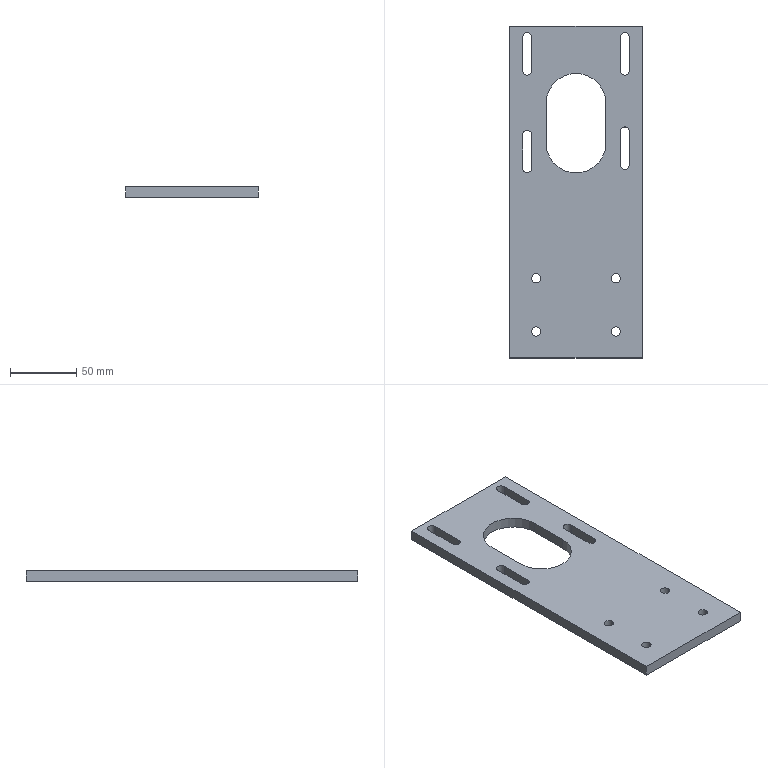Part | STEP file | AC motor fixing | 1 solid | 34 faces | box 100 x 250 x 8 mm | volume 168414 mm3 | cylinder 18 | plane 16 | commonest cylinder face diameters 7 x16 45 x2
STEP:
#1=CARTESIAN_POINT('',(83.5,-230.,8.));
#2=VERTEX_POINT('',#1);
#3=CARTESIAN_POINT('',(76.5,-230.,8.));
#4=VERTEX_POINT('',#3);
#5=CARTESIAN_POINT('',(80.,-230.,8.));
#6=DIRECTION('',(0.,0.,-1.));
#7=DIRECTION('',(1.,0.,0.));
#8=AXIS2_PLACEMENT_3D('',#5,#6,#7);
#9=CIRCLE('',#8,3.5);
#10=EDGE_CURVE('',#2,#4,#9,.T.);
#11=ORIENTED_EDGE('',*,*,#10,.F.);
#12=CARTESIAN_POINT('',(83.5,-230.,0.));
#13=VERTEX_POINT('',#12);
#14=CARTESIAN_POINT('',(83.5,-230.,8.));
#15=DIRECTION('',(0.,0.,-1.));
#16=VECTOR('',#15,1000.);
#17=LINE('',#14,#16);
#18=EDGE_CURVE('',#2,#13,#17,.T.);
#19=ORIENTED_EDGE('',*,*,#18,.T.);
#20=CARTESIAN_POINT('',(76.5,-230.,0.));
#21=VERTEX_POINT('',#20);
#22=CARTESIAN_POINT('',(80.,-230.,0.));
#23=DIRECTION('',(0.,0.,-1.));
#24=DIRECTION('',(1.,0.,0.));
#25=AXIS2_PLACEMENT_3D('',#22,#23,#24);
#26=CIRCLE('',#25,3.5);
#27=EDGE_CURVE('',#13,#21,#26,.T.);
#28=ORIENTED_EDGE('',*,*,#27,.T.);
#29=CARTESIAN_POINT('',(76.5,-230.,8.));
#30=DIRECTION('',(0.,0.,-1.));
#31=VECTOR('',#30,1000.);
#32=LINE('',#29,#31);
#33=EDGE_CURVE('',#4,#21,#32,.T.);
#34=ORIENTED_EDGE('',*,*,#33,.F.);
#35=EDGE_LOOP('',(#11,#19,#28,#34));
#36=FACE_OUTER_BOUND('',#35,.T.);
#37=CARTESIAN_POINT('',(80.,-230.,8.));
#38=DIRECTION('',(0.,0.,-1.));
#39=DIRECTION('',(-1.,0.,0.));
#40=AXIS2_PLACEMENT_3D('',#37,#38,#39);
#41=CYLINDRICAL_SURFACE('',#40,3.5);
#42=ADVANCED_FACE('',(#36),#41,.F.);
#43=CARTESIAN_POINT('',(23.5,-190.,8.));
#44=VERTEX_POINT('',#43);
#45=CARTESIAN_POINT('',(16.5,-190.,8.));
#46=VERTEX_POINT('',#45);
#47=CARTESIAN_POINT('',(20.,-190.,8.));
#48=DIRECTION('',(0.,0.,-1.));
#49=DIRECTION('',(-1.,0.,0.));
#50=AXIS2_PLACEMENT_3D('',#47,#48,#49);
#51=CIRCLE('',#50,3.5);
#52=EDGE_CURVE('',#44,#46,#51,.T.);
#53=ORIENTED_EDGE('',*,*,#52,.F.);
#54=CARTESIAN_POINT('',(23.5,-190.,0.));
#55=VERTEX_POINT('',#54);
#56=CARTESIAN_POINT('',(23.5,-190.,8.));
#57=DIRECTION('',(0.,0.,-1.));
#58=VECTOR('',#57,1000.);
#59=LINE('',#56,#58);
#60=EDGE_CURVE('',#44,#55,#59,.T.);
#61=ORIENTED_EDGE('',*,*,#60,.T.);
#62=CARTESIAN_POINT('',(16.5,-190.,0.));
#63=VERTEX_POINT('',#62);
#64=CARTESIAN_POINT('',(20.,-190.,0.));
#65=DIRECTION('',(0.,0.,-1.));
#66=DIRECTION('',(-1.,0.,0.));
#67=AXIS2_PLACEMENT_3D('',#64,#65,#66);
#68=CIRCLE('',#67,3.5);
#69=EDGE_CURVE('',#55,#63,#68,.T.);
#70=ORIENTED_EDGE('',*,*,#69,.T.);
#71=CARTESIAN_POINT('',(16.5,-190.,8.));
#72=DIRECTION('',(0.,0.,-1.));
#73=VECTOR('',#72,1000.);
#74=LINE('',#71,#73);
#75=EDGE_CURVE('',#46,#63,#74,.T.);
#76=ORIENTED_EDGE('',*,*,#75,.F.);
#77=EDGE_LOOP('',(#53,#61,#70,#76));
#78=FACE_OUTER_BOUND('',#77,.T.);
#79=CARTESIAN_POINT('',(20.,-190.,8.));
#80=DIRECTION('',(0.,0.,-1.));
#81=DIRECTION('',(-1.,0.,0.));
#82=AXIS2_PLACEMENT_3D('',#79,#80,#81);
#83=CYLINDRICAL_SURFACE('',#82,3.5);
#84=ADVANCED_FACE('',(#78),#83,.F.);
#85=CARTESIAN_POINT('',(83.5,-190.,8.));
#86=VERTEX_POINT('',#85);
#87=CARTESIAN_POINT('',(76.5,-190.,8.));
#88=VERTEX_POINT('',#87);
#89=CARTESIAN_POINT('',(80.,-190.,8.));
#90=DIRECTION('',(0.,0.,-1.));
#91=DIRECTION('',(1.,0.,0.));
#92=AXIS2_PLACEMENT_3D('',#89,#90,#91);
#93=CIRCLE('',#92,3.5);
#94=EDGE_CURVE('',#86,#88,#93,.T.);
#95=ORIENTED_EDGE('',*,*,#94,.F.);
#96=CARTESIAN_POINT('',(83.5,-190.,0.));
#97=VERTEX_POINT('',#96);
#98=CARTESIAN_POINT('',(83.5,-190.,8.));
#99=DIRECTION('',(0.,0.,-1.));
#100=VECTOR('',#99,1000.);
#101=LINE('',#98,#100);
#102=EDGE_CURVE('',#86,#97,#101,.T.);
#103=ORIENTED_EDGE('',*,*,#102,.T.);
#104=CARTESIAN_POINT('',(76.5,-190.,0.));
#105=VERTEX_POINT('',#104);
#106=CARTESIAN_POINT('',(80.,-190.,0.));
#107=DIRECTION('',(0.,0.,-1.));
#108=DIRECTION('',(1.,0.,0.));
#109=AXIS2_PLACEMENT_3D('',#106,#107,#108);
#110=CIRCLE('',#109,3.5);
#111=EDGE_CURVE('',#97,#105,#110,.T.);
#112=ORIENTED_EDGE('',*,*,#111,.T.);
#113=CARTESIAN_POINT('',(76.5,-190.,8.));
#114=DIRECTION('',(0.,0.,-1.));
#115=VECTOR('',#114,1000.);
#116=LINE('',#113,#115);
#117=EDGE_CURVE('',#88,#105,#116,.T.);
#118=ORIENTED_EDGE('',*,*,#117,.F.);
#119=EDGE_LOOP('',(#95,#103,#112,#118));
#120=FACE_OUTER_BOUND('',#119,.T.);
#121=CARTESIAN_POINT('',(80.,-190.,8.));
#122=DIRECTION('',(0.,0.,-1.));
#123=DIRECTION('',(-1.,0.,0.));
#124=AXIS2_PLACEMENT_3D('',#121,#122,#123);
#125=CYLINDRICAL_SURFACE('',#124,3.5);
#126=ADVANCED_FACE('',(#120),#125,.F.);
#127=CARTESIAN_POINT('',(23.5,-230.,8.));
#128=VERTEX_POINT('',#127);
#129=CARTESIAN_POINT('',(16.5,-230.,8.));
#130=VERTEX_POINT('',#129);
#131=CARTESIAN_POINT('',(20.,-230.,8.));
#132=DIRECTION('',(0.,0.,-1.));
#133=DIRECTION('',(-1.,0.,0.));
#134=AXIS2_PLACEMENT_3D('',#131,#132,#133);
#135=CIRCLE('',#134,3.5);
#136=EDGE_CURVE('',#128,#130,#135,.T.);
#137=ORIENTED_EDGE('',*,*,#136,.F.);
#138=CARTESIAN_POINT('',(23.5,-230.,0.));
#139=VERTEX_POINT('',#138);
#140=CARTESIAN_POINT('',(23.5,-230.,8.));
#141=DIRECTION('',(0.,0.,-1.));
#142=VECTOR('',#141,1000.);
#143=LINE('',#140,#142);
#144=EDGE_CURVE('',#128,#139,#143,.T.);
#145=ORIENTED_EDGE('',*,*,#144,.T.);
#146=CARTESIAN_POINT('',(16.5,-230.,0.));
#147=VERTEX_POINT('',#146);
#148=CARTESIAN_POINT('',(20.,-230.,0.));
#149=DIRECTION('',(0.,0.,-1.));
#150=DIRECTION('',(-1.,0.,0.));
#151=AXIS2_PLACEMENT_3D('',#148,#149,#150);
#152=CIRCLE('',#151,3.5);
#153=EDGE_CURVE('',#139,#147,#152,.T.);
#154=ORIENTED_EDGE('',*,*,#153,.T.);
#155=CARTESIAN_POINT('',(16.5,-230.,8.));
#156=DIRECTION('',(0.,0.,-1.));
#157=VECTOR('',#156,1000.);
#158=LINE('',#155,#157);
#159=EDGE_CURVE('',#130,#147,#158,.T.);
#160=ORIENTED_EDGE('',*,*,#159,.F.);
#161=EDGE_LOOP('',(#137,#145,#154,#160));
#162=FACE_OUTER_BOUND('',#161,.T.);
#163=CARTESIAN_POINT('',(20.,-230.,8.));
#164=DIRECTION('',(0.,0.,-1.));
#165=DIRECTION('',(-1.,0.,0.));
#166=AXIS2_PLACEMENT_3D('',#163,#164,#165);
#167=CYLINDRICAL_SURFACE('',#166,3.5);
#168=ADVANCED_FACE('',(#162),#167,.F.);
#169=CARTESIAN_POINT('',(0.,0.,0.));
#170=VERTEX_POINT('',#169);
#171=CARTESIAN_POINT('',(0.,-250.,0.));
#172=VERTEX_POINT('',#171);
#173=CARTESIAN_POINT('',(0.,0.,0.));
#174=DIRECTION('',(0.,-1.,0.));
#175=VECTOR('',#174,1000.);
#176=LINE('',#173,#175);
#177=EDGE_CURVE('',#170,#172,#176,.T.);
#178=ORIENTED_EDGE('',*,*,#177,.T.);
#179=CARTESIAN_POINT('',(0.,-250.,8.));
#180=VERTEX_POINT('',#179);
#181=CARTESIAN_POINT('',(0.,-250.,8.));
#182=DIRECTION('',(0.,0.,-1.));
#183=VECTOR('',#182,1000.);
#184=LINE('',#181,#183);
#185=EDGE_CURVE('',#180,#172,#184,.T.);
#186=ORIENTED_EDGE('',*,*,#185,.F.);
#187=CARTESIAN_POINT('',(0.,0.,8.));
#188=VERTEX_POINT('',#187);
#189=CARTESIAN_POINT('',(0.,0.,8.));
#190=DIRECTION('',(0.,-1.,0.));
#191=VECTOR('',#190,1000.);
#192=LINE('',#189,#191);
#193=EDGE_CURVE('',#188,#180,#192,.T.);
#194=ORIENTED_EDGE('',*,*,#193,.F.);
#195=CARTESIAN_POINT('',(0.,0.,8.));
#196=DIRECTION('',(0.,0.,-1.));
#197=VECTOR('',#196,1000.);
#198=LINE('',#195,#197);
#199=EDGE_CURVE('',#188,#170,#198,.T.);
#200=ORIENTED_EDGE('',*,*,#199,.T.);
#201=EDGE_LOOP('',(#178,#186,#194,#200));
#202=FACE_OUTER_BOUND('',#201,.T.);
#203=CARTESIAN_POINT('',(0.,0.,8.));
#204=DIRECTION('',(1.,0.,0.));
#205=DIRECTION('',(0.,1.,0.));
#206=AXIS2_PLACEMENT_3D('',#203,#204,#205);
#207=PLANE('',#206);
#208=ADVANCED_FACE('',(#202),#207,.F.);
#209=CARTESIAN_POINT('',(100.,-250.,0.));
#210=VERTEX_POINT('',#209);
#211=CARTESIAN_POINT('',(0.,-250.,0.));
#212=DIRECTION('',(1.,0.,0.));
#213=VECTOR('',#212,1000.);
#214=LINE('',#211,#213);
#215=EDGE_CURVE('',#172,#210,#214,.T.);
#216=ORIENTED_EDGE('',*,*,#215,.T.);
#217=CARTESIAN_POINT('',(100.,-250.,8.));
#218=VERTEX_POINT('',#217);
#219=CARTESIAN_POINT('',(100.,-250.,8.));
#220=DIRECTION('',(0.,0.,-1.));
#221=VECTOR('',#220,1000.);
#222=LINE('',#219,#221);
#223=EDGE_CURVE('',#218,#210,#222,.T.);
#224=ORIENTED_EDGE('',*,*,#223,.F.);
#225=CARTESIAN_POINT('',(0.,-250.,8.));
#226=DIRECTION('',(1.,0.,0.));
#227=VECTOR('',#226,1000.);
#228=LINE('',#225,#227);
#229=EDGE_CURVE('',#180,#218,#228,.T.);
#230=ORIENTED_EDGE('',*,*,#229,.F.);
#231=ORIENTED_EDGE('',*,*,#185,.T.);
#232=EDGE_LOOP('',(#216,#224,#230,#231));
#233=FACE_OUTER_BOUND('',#232,.T.);
#234=CARTESIAN_POINT('',(0.,-250.,8.));
#235=DIRECTION('',(0.,1.,0.));
#236=DIRECTION('',(0.,0.,1.));
#237=AXIS2_PLACEMENT_3D('',#234,#235,#236);
#238=PLANE('',#237);
#239=ADVANCED_FACE('',(#233),#238,.F.);
#240=CARTESIAN_POINT('',(100.,0.,0.));
#241=VERTEX_POINT('',#240);
#242=CARTESIAN_POINT('',(100.,0.,0.));
#243=DIRECTION('',(0.,1.,0.));
#244=VECTOR('',#243,1000.);
#245=LINE('',#242,#244);
#246=EDGE_CURVE('',#210,#241,#245,.T.);
#247=ORIENTED_EDGE('',*,*,#246,.T.);
#248=CARTESIAN_POINT('',(100.,0.,8.));
#249=VERTEX_POINT('',#248);
#250=CARTESIAN_POINT('',(100.,0.,8.));
#251=DIRECTION('',(0.,0.,-1.));
#252=VECTOR('',#251,1000.);
#253=LINE('',#250,#252);
#254=EDGE_CURVE('',#249,#241,#253,.T.);
#255=ORIENTED_EDGE('',*,*,#254,.F.);
#256=CARTESIAN_POINT('',(100.,0.,8.));
#257=DIRECTION('',(0.,1.,0.));
#258=VECTOR('',#257,1000.);
#259=LINE('',#256,#258);
#260=EDGE_CURVE('',#218,#249,#259,.T.);
#261=ORIENTED_EDGE('',*,*,#260,.F.);
#262=ORIENTED_EDGE('',*,*,#223,.T.);
#263=EDGE_LOOP('',(#247,#255,#261,#262));
#264=FACE_OUTER_BOUND('',#263,.T.);
#265=CARTESIAN_POINT('',(100.,0.,8.));
#266=DIRECTION('',(-1.,0.,0.));
#267=DIRECTION('',(0.,-1.,0.));
#268=AXIS2_PLACEMENT_3D('',#265,#266,#267);
#269=PLANE('',#268);
#270=ADVANCED_FACE('',(#264),#269,.F.);
#271=CARTESIAN_POINT('',(0.,0.,0.));
#272=DIRECTION('',(-1.,0.,0.));
#273=VECTOR('',#272,1000.);
#274=LINE('',#271,#273);
#275=EDGE_CURVE('',#241,#170,#274,.T.);
#276=ORIENTED_EDGE('',*,*,#275,.T.);
#277=ORIENTED_EDGE('',*,*,#199,.F.);
#278=CARTESIAN_POINT('',(0.,0.,8.));
#279=DIRECTION('',(-1.,0.,0.));
#280=VECTOR('',#279,1000.);
#281=LINE('',#278,#280);
#282=EDGE_CURVE('',#249,#188,#281,.T.);
#283=ORIENTED_EDGE('',*,*,#282,.F.);
#284=ORIENTED_EDGE('',*,*,#254,.T.);
#285=EDGE_LOOP('',(#276,#277,#283,#284));
#286=FACE_OUTER_BOUND('',#285,.T.);
#287=CARTESIAN_POINT('',(0.,0.,8.));
#288=DIRECTION('',(0.,-1.,0.));
#289=DIRECTION('',(0.,0.,-1.));
#290=AXIS2_PLACEMENT_3D('',#287,#288,#289);
#291=PLANE('',#290);
#292=ADVANCED_FACE('',(#286),#291,.F.);
#293=CARTESIAN_POINT('',(80.,-230.,8.));
#294=DIRECTION('',(0.,0.,-1.));
#295=DIRECTION('',(1.,0.,0.));
#296=AXIS2_PLACEMENT_3D('',#293,#294,#295);
#297=CIRCLE('',#296,3.5);
#298=EDGE_CURVE('',#4,#2,#297,.T.);
#299=ORIENTED_EDGE('',*,*,#298,.T.);
#300=ORIENTED_EDGE('',*,*,#10,.T.);
#301=EDGE_LOOP('',(#299,#300));
#302=FACE_BOUND('',#301,.T.);
#303=CARTESIAN_POINT('',(20.,-190.,8.));
#304=DIRECTION('',(0.,0.,-1.));
#305=DIRECTION('',(-1.,0.,0.));
#306=AXIS2_PLACEMENT_3D('',#303,#304,#305);
#307=CIRCLE('',#306,3.5);
#308=EDGE_CURVE('',#46,#44,#307,.T.);
#309=ORIENTED_EDGE('',*,*,#308,.T.);
#310=ORIENTED_EDGE('',*,*,#52,.T.);
#311=EDGE_LOOP('',(#309,#310));
#312=FACE_BOUND('',#311,.T.);
#313=CARTESIAN_POINT('',(80.,-190.,8.));
#314=DIRECTION('',(0.,0.,-1.));
#315=DIRECTION('',(1.,0.,0.));
#316=AXIS2_PLACEMENT_3D('',#313,#314,#315);
#317=CIRCLE('',#316,3.5);
#318=EDGE_CURVE('',#88,#86,#317,.T.);
#319=ORIENTED_EDGE('',*,*,#318,.T.);
#320=ORIENTED_EDGE('',*,*,#94,.T.);
#321=EDGE_LOOP('',(#319,#320));
#322=FACE_BOUND('',#321,.T.);
#323=CARTESIAN_POINT('',(20.,-230.,8.));
#324=DIRECTION('',(0.,0.,-1.));
#325=DIRECTION('',(-1.,0.,0.));
#326=AXIS2_PLACEMENT_3D('',#323,#324,#325);
#327=CIRCLE('',#326,3.5);
#328=EDGE_CURVE('',#130,#128,#327,.T.);
#329=ORIENTED_EDGE('',*,*,#328,.T.);
#330=ORIENTED_EDGE('',*,*,#136,.T.);
#331=EDGE_LOOP('',(#329,#330));
#332=FACE_BOUND('',#331,.T.);
#333=CARTESIAN_POINT('',(27.5,-58.25,8.));
#334=VERTEX_POINT('',#333);
#335=CARTESIAN_POINT('',(72.5,-58.25,8.));
#336=VERTEX_POINT('',#335);
#337=CARTESIAN_POINT('',(50.,-58.25,8.));
#338=DIRECTION('',(0.,0.,-1.));
#339=DIRECTION('',(-1.,0.,0.));
#340=AXIS2_PLACEMENT_3D('',#337,#338,#339);
#341=CIRCLE('',#340,22.5);
#342=EDGE_CURVE('',#334,#336,#341,.T.);
#343=ORIENTED_EDGE('',*,*,#342,.T.);
#344=CARTESIAN_POINT('',(72.5,-88.25,8.));
#345=VERTEX_POINT('',#344);
#346=CARTESIAN_POINT('',(72.5,-58.25,8.));
#347=DIRECTION('',(0.,-1.,0.));
#348=VECTOR('',#347,1000.);
#349=LINE('',#346,#348);
#350=EDGE_CURVE('',#336,#345,#349,.T.);
#351=ORIENTED_EDGE('',*,*,#350,.T.);
#352=CARTESIAN_POINT('',(27.5,-88.25,8.));
#353=VERTEX_POINT('',#352);
#354=CARTESIAN_POINT('',(50.,-88.25,8.));
#355=DIRECTION('',(0.,0.,-1.));
#356=DIRECTION('',(-1.,0.,0.));
#357=AXIS2_PLACEMENT_3D('',#354,#355,#356);
#358=CIRCLE('',#357,22.5);
#359=EDGE_CURVE('',#345,#353,#358,.T.);
#360=ORIENTED_EDGE('',*,*,#359,.T.);
#361=CARTESIAN_POINT('',(27.5,-58.25,8.));
#362=DIRECTION('',(0.,1.,0.));
#363=VECTOR('',#362,1000.);
#364=LINE('',#361,#363);
#365=EDGE_CURVE('',#353,#334,#364,.T.);
#366=ORIENTED_EDGE('',*,*,#365,.T.);
#367=EDGE_LOOP('',(#343,#351,#360,#366));
#368=FACE_BOUND('',#367,.T.);
#369=CARTESIAN_POINT('',(9.73,-82.02,8.));
#370=VERTEX_POINT('',#369);
#371=CARTESIAN_POINT('',(16.73,-82.02,8.));
#372=VERTEX_POINT('',#371);
#373=CARTESIAN_POINT('',(13.23,-82.02,8.));
#374=DIRECTION('',(0.,0.,-1.));
#375=DIRECTION('',(-1.,0.,0.));
#376=AXIS2_PLACEMENT_3D('',#373,#374,#375);
#377=CIRCLE('',#376,3.5);
#378=EDGE_CURVE('',#370,#372,#377,.T.);
#379=ORIENTED_EDGE('',*,*,#378,.T.);
#380=CARTESIAN_POINT('',(16.73,-107.02,8.));
#381=VERTEX_POINT('',#380);
#382=CARTESIAN_POINT('',(16.73,-82.02,8.));
#383=DIRECTION('',(0.,-1.,0.));
#384=VECTOR('',#383,1000.);
#385=LINE('',#382,#384);
#386=EDGE_CURVE('',#372,#381,#385,.T.);
#387=ORIENTED_EDGE('',*,*,#386,.T.);
#388=CARTESIAN_POINT('',(9.73,-107.02,8.));
#389=VERTEX_POINT('',#388);
#390=CARTESIAN_POINT('',(13.23,-107.02,8.));
#391=DIRECTION('',(0.,0.,-1.));
#392=DIRECTION('',(-1.,0.,0.));
#393=AXIS2_PLACEMENT_3D('',#390,#391,#392);
#394=CIRCLE('',#393,3.5);
#395=EDGE_CURVE('',#381,#389,#394,.T.);
#396=ORIENTED_EDGE('',*,*,#395,.T.);
#397=CARTESIAN_POINT('',(9.73,-82.02,8.));
#398=DIRECTION('',(0.,1.,0.));
#399=VECTOR('',#398,1000.);
#400=LINE('',#397,#399);
#401=EDGE_CURVE('',#389,#370,#400,.T.);
#402=ORIENTED_EDGE('',*,*,#401,.T.);
#403=EDGE_LOOP('',(#379,#387,#396,#402));
#404=FACE_BOUND('',#403,.T.);
#405=CARTESIAN_POINT('',(9.73,-8.48,8.));
#406=VERTEX_POINT('',#405);
#407=CARTESIAN_POINT('',(16.73,-8.48,8.));
#408=VERTEX_POINT('',#407);
#409=CARTESIAN_POINT('',(13.23,-8.48,8.));
#410=DIRECTION('',(0.,0.,-1.));
#411=DIRECTION('',(-1.,0.,0.));
#412=AXIS2_PLACEMENT_3D('',#409,#410,#411);
#413=CIRCLE('',#412,3.5);
#414=EDGE_CURVE('',#406,#408,#413,.T.);
#415=ORIENTED_EDGE('',*,*,#414,.T.);
#416=CARTESIAN_POINT('',(16.73,-33.48,8.));
#417=VERTEX_POINT('',#416);
#418=CARTESIAN_POINT('',(16.73,-8.48,8.));
#419=DIRECTION('',(0.,-1.,0.));
#420=VECTOR('',#419,1000.);
#421=LINE('',#418,#420);
#422=EDGE_CURVE('',#408,#417,#421,.T.);
#423=ORIENTED_EDGE('',*,*,#422,.T.);
#424=CARTESIAN_POINT('',(9.73,-33.48,8.));
#425=VERTEX_POINT('',#424);
#426=CARTESIAN_POINT('',(13.23,-33.48,8.));
#427=DIRECTION('',(0.,0.,-1.));
#428=DIRECTION('',(-1.,0.,0.));
#429=AXIS2_PLACEMENT_3D('',#426,#427,#428);
#430=CIRCLE('',#429,3.5);
#431=EDGE_CURVE('',#417,#425,#430,.T.);
#432=ORIENTED_EDGE('',*,*,#431,.T.);
#433=CARTESIAN_POINT('',(9.73,-8.48,8.));
#434=DIRECTION('',(0.,1.,0.));
#435=VECTOR('',#434,1000.);
#436=LINE('',#433,#435);
#437=EDGE_CURVE('',#425,#406,#436,.T.);
#438=ORIENTED_EDGE('',*,*,#437,.T.);
#439=EDGE_LOOP('',(#415,#423,#432,#438));
#440=FACE_BOUND('',#439,.T.);
#441=CARTESIAN_POINT('',(83.27,-8.48,8.));
#442=VERTEX_POINT('',#441);
#443=CARTESIAN_POINT('',(90.27,-8.48,8.));
#444=VERTEX_POINT('',#443);
#445=CARTESIAN_POINT('',(86.77,-8.48,8.));
#446=DIRECTION('',(0.,0.,-1.));
#447=DIRECTION('',(-1.,0.,0.));
#448=AXIS2_PLACEMENT_3D('',#445,#446,#447);
#449=CIRCLE('',#448,3.5);
#450=EDGE_CURVE('',#442,#444,#449,.T.);
#451=ORIENTED_EDGE('',*,*,#450,.T.);
#452=CARTESIAN_POINT('',(90.27,-33.48,8.));
#453=VERTEX_POINT('',#452);
#454=CARTESIAN_POINT('',(90.27,-8.48,8.));
#455=DIRECTION('',(0.,-1.,0.));
#456=VECTOR('',#455,1000.);
#457=LINE('',#454,#456);
#458=EDGE_CURVE('',#444,#453,#457,.T.);
#459=ORIENTED_EDGE('',*,*,#458,.T.);
#460=CARTESIAN_POINT('',(83.27,-33.48,8.));
#461=VERTEX_POINT('',#460);
#462=CARTESIAN_POINT('',(86.77,-33.48,8.));
#463=DIRECTION('',(0.,0.,-1.));
#464=DIRECTION('',(-1.,0.,0.));
#465=AXIS2_PLACEMENT_3D('',#462,#463,#464);
#466=CIRCLE('',#465,3.5);
#467=EDGE_CURVE('',#453,#461,#466,.T.);
#468=ORIENTED_EDGE('',*,*,#467,.T.);
#469=CARTESIAN_POINT('',(83.27,-8.48,8.));
#470=DIRECTION('',(0.,1.,0.));
#471=VECTOR('',#470,1000.);
#472=LINE('',#469,#471);
#473=EDGE_CURVE('',#461,#442,#472,.T.);
#474=ORIENTED_EDGE('',*,*,#473,.T.);
#475=EDGE_LOOP('',(#451,#459,#468,#474));
#476=FACE_BOUND('',#475,.T.);
#477=CARTESIAN_POINT('',(83.27,-79.52,8.));
#478=VERTEX_POINT('',#477);
#479=CARTESIAN_POINT('',(90.27,-79.52,8.));
#480=VERTEX_POINT('',#479);
#481=CARTESIAN_POINT('',(86.77,-79.52,8.));
#482=DIRECTION('',(0.,0.,-1.));
#483=DIRECTION('',(-1.,0.,0.));
#484=AXIS2_PLACEMENT_3D('',#481,#482,#483);
#485=CIRCLE('',#484,3.5);
#486=EDGE_CURVE('',#478,#480,#485,.T.);
#487=ORIENTED_EDGE('',*,*,#486,.T.);
#488=CARTESIAN_POINT('',(90.27,-104.52,8.));
#489=VERTEX_POINT('',#488);
#490=CARTESIAN_POINT('',(90.27,-79.52,8.));
#491=DIRECTION('',(0.,-1.,0.));
#492=VECTOR('',#491,1000.);
#493=LINE('',#490,#492);
#494=EDGE_CURVE('',#480,#489,#493,.T.);
#495=ORIENTED_EDGE('',*,*,#494,.T.);
#496=CARTESIAN_POINT('',(83.27,-104.52,8.));
#497=VERTEX_POINT('',#496);
#498=CARTESIAN_POINT('',(86.77,-104.52,8.));
#499=DIRECTION('',(0.,0.,-1.));
#500=DIRECTION('',(-1.,0.,0.));
#501=AXIS2_PLACEMENT_3D('',#498,#499,#500);
#502=CIRCLE('',#501,3.5);
#503=EDGE_CURVE('',#489,#497,#502,.T.);
#504=ORIENTED_EDGE('',*,*,#503,.T.);
#505=CARTESIAN_POINT('',(83.27,-79.52,8.));
#506=DIRECTION('',(0.,1.,0.));
#507=VECTOR('',#506,1000.);
#508=LINE('',#505,#507);
#509=EDGE_CURVE('',#497,#478,#508,.T.);
#510=ORIENTED_EDGE('',*,*,#509,.T.);
#511=EDGE_LOOP('',(#487,#495,#504,#510));
#512=FACE_BOUND('',#511,.T.);
#513=ORIENTED_EDGE('',*,*,#193,.T.);
#514=ORIENTED_EDGE('',*,*,#229,.T.);
#515=ORIENTED_EDGE('',*,*,#260,.T.);
#516=ORIENTED_EDGE('',*,*,#282,.T.);
#517=EDGE_LOOP('',(#513,#514,#515,#516));
#518=FACE_OUTER_BOUND('',#517,.T.);
#519=CARTESIAN_POINT('',(0.,0.,8.));
#520=DIRECTION('',(0.,0.,1.));
#521=DIRECTION('',(1.,0.,0.));
#522=AXIS2_PLACEMENT_3D('',#519,#520,#521);
#523=PLANE('',#522);
#524=ADVANCED_FACE('',(#302,#312,#322,#332,#368,#404,#440,#476,#512,#518),#523,.T.);
#525=CARTESIAN_POINT('',(80.,-230.,0.));
#526=DIRECTION('',(0.,0.,-1.));
#527=DIRECTION('',(1.,0.,0.));
#528=AXIS2_PLACEMENT_3D('',#525,#526,#527);
#529=CIRCLE('',#528,3.5);
#530=EDGE_CURVE('',#21,#13,#529,.T.);
#531=ORIENTED_EDGE('',*,*,#530,.F.);
#532=ORIENTED_EDGE('',*,*,#27,.F.);
#533=EDGE_LOOP('',(#531,#532));
#534=FACE_BOUND('',#533,.T.);
#535=CARTESIAN_POINT('',(20.,-190.,0.));
#536=DIRECTION('',(0.,0.,-1.));
#537=DIRECTION('',(-1.,0.,0.));
#538=AXIS2_PLACEMENT_3D('',#535,#536,#537);
#539=CIRCLE('',#538,3.5);
#540=EDGE_CURVE('',#63,#55,#539,.T.);
#541=ORIENTED_EDGE('',*,*,#540,.F.);
#542=ORIENTED_EDGE('',*,*,#69,.F.);
#543=EDGE_LOOP('',(#541,#542));
#544=FACE_BOUND('',#543,.T.);
#545=CARTESIAN_POINT('',(80.,-190.,0.));
#546=DIRECTION('',(0.,0.,-1.));
#547=DIRECTION('',(1.,0.,0.));
#548=AXIS2_PLACEMENT_3D('',#545,#546,#547);
#549=CIRCLE('',#548,3.5);
#550=EDGE_CURVE('',#105,#97,#549,.T.);
#551=ORIENTED_EDGE('',*,*,#550,.F.);
#552=ORIENTED_EDGE('',*,*,#111,.F.);
#553=EDGE_LOOP('',(#551,#552));
#554=FACE_BOUND('',#553,.T.);
#555=CARTESIAN_POINT('',(20.,-230.,0.));
#556=DIRECTION('',(0.,0.,-1.));
#557=DIRECTION('',(-1.,0.,0.));
#558=AXIS2_PLACEMENT_3D('',#555,#556,#557);
#559=CIRCLE('',#558,3.5);
#560=EDGE_CURVE('',#147,#139,#559,.T.);
#561=ORIENTED_EDGE('',*,*,#560,.F.);
#562=ORIENTED_EDGE('',*,*,#153,.F.);
#563=EDGE_LOOP('',(#561,#562));
#564=FACE_BOUND('',#563,.T.);
#565=CARTESIAN_POINT('',(16.73,-82.02,0.));
#566=VERTEX_POINT('',#565);
#567=CARTESIAN_POINT('',(16.73,-107.02,0.));
#568=VERTEX_POINT('',#567);
#569=CARTESIAN_POINT('',(16.73,-82.02,0.));
#570=DIRECTION('',(0.,-1.,0.));
#571=VECTOR('',#570,1000.);
#572=LINE('',#569,#571);
#573=EDGE_CURVE('',#566,#568,#572,.T.);
#574=ORIENTED_EDGE('',*,*,#573,.F.);
#575=CARTESIAN_POINT('',(9.73,-82.02,0.));
#576=VERTEX_POINT('',#575);
#577=CARTESIAN_POINT('',(13.23,-82.02,0.));
#578=DIRECTION('',(0.,0.,-1.));
#579=DIRECTION('',(-1.,0.,0.));
#580=AXIS2_PLACEMENT_3D('',#577,#578,#579);
#581=CIRCLE('',#580,3.5);
#582=EDGE_CURVE('',#576,#566,#581,.T.);
#583=ORIENTED_EDGE('',*,*,#582,.F.);
#584=CARTESIAN_POINT('',(9.73,-107.02,0.));
#585=VERTEX_POINT('',#584);
#586=CARTESIAN_POINT('',(9.73,-82.02,0.));
#587=DIRECTION('',(0.,1.,0.));
#588=VECTOR('',#587,1000.);
#589=LINE('',#586,#588);
#590=EDGE_CURVE('',#585,#576,#589,.T.);
#591=ORIENTED_EDGE('',*,*,#590,.F.);
#592=CARTESIAN_POINT('',(13.23,-107.02,0.));
#593=DIRECTION('',(0.,0.,-1.));
#594=DIRECTION('',(-1.,0.,0.));
#595=AXIS2_PLACEMENT_3D('',#592,#593,#594);
#596=CIRCLE('',#595,3.5);
#597=EDGE_CURVE('',#568,#585,#596,.T.);
#598=ORIENTED_EDGE('',*,*,#597,.F.);
#599=EDGE_LOOP('',(#574,#583,#591,#598));
#600=FACE_BOUND('',#599,.T.);
#601=CARTESIAN_POINT('',(16.73,-8.48,0.));
#602=VERTEX_POINT('',#601);
#603=CARTESIAN_POINT('',(16.73,-33.48,0.));
#604=VERTEX_POINT('',#603);
#605=CARTESIAN_POINT('',(16.73,-8.48,0.));
#606=DIRECTION('',(0.,-1.,0.));
#607=VECTOR('',#606,1000.);
#608=LINE('',#605,#607);
#609=EDGE_CURVE('',#602,#604,#608,.T.);
#610=ORIENTED_EDGE('',*,*,#609,.F.);
#611=CARTESIAN_POINT('',(9.73,-8.48,0.));
#612=VERTEX_POINT('',#611);
#613=CARTESIAN_POINT('',(13.23,-8.48,0.));
#614=DIRECTION('',(0.,0.,-1.));
#615=DIRECTION('',(-1.,0.,0.));
#616=AXIS2_PLACEMENT_3D('',#613,#614,#615);
#617=CIRCLE('',#616,3.5);
#618=EDGE_CURVE('',#612,#602,#617,.T.);
#619=ORIENTED_EDGE('',*,*,#618,.F.);
#620=CARTESIAN_POINT('',(9.73,-33.48,0.));
#621=VERTEX_POINT('',#620);
#622=CARTESIAN_POINT('',(9.73,-8.48,0.));
#623=DIRECTION('',(0.,1.,0.));
#624=VECTOR('',#623,1000.);
#625=LINE('',#622,#624);
#626=EDGE_CURVE('',#621,#612,#625,.T.);
#627=ORIENTED_EDGE('',*,*,#626,.F.);
#628=CARTESIAN_POINT('',(13.23,-33.48,0.));
#629=DIRECTION('',(0.,0.,-1.));
#630=DIRECTION('',(-1.,0.,0.));
#631=AXIS2_PLACEMENT_3D('',#628,#629,#630);
#632=CIRCLE('',#631,3.5);
#633=EDGE_CURVE('',#604,#621,#632,.T.);
#634=ORIENTED_EDGE('',*,*,#633,.F.);
#635=EDGE_LOOP('',(#610,#619,#627,#634));
#636=FACE_BOUND('',#635,.T.);
#637=CARTESIAN_POINT('',(90.27,-8.48,0.));
#638=VERTEX_POINT('',#637);
#639=CARTESIAN_POINT('',(90.27,-33.48,0.));
#640=VERTEX_POINT('',#639);
#641=CARTESIAN_POINT('',(90.27,-8.48,0.));
#642=DIRECTION('',(0.,-1.,0.));
#643=VECTOR('',#642,1000.);
#644=LINE('',#641,#643);
#645=EDGE_CURVE('',#638,#640,#644,.T.);
#646=ORIENTED_EDGE('',*,*,#645,.F.);
#647=CARTESIAN_POINT('',(83.27,-8.48,0.));
#648=VERTEX_POINT('',#647);
#649=CARTESIAN_POINT('',(86.77,-8.48,0.));
#650=DIRECTION('',(0.,0.,-1.));
#651=DIRECTION('',(-1.,0.,0.));
#652=AXIS2_PLACEMENT_3D('',#649,#650,#651);
#653=CIRCLE('',#652,3.5);
#654=EDGE_CURVE('',#648,#638,#653,.T.);
#655=ORIENTED_EDGE('',*,*,#654,.F.);
#656=CARTESIAN_POINT('',(83.27,-33.48,0.));
#657=VERTEX_POINT('',#656);
#658=CARTESIAN_POINT('',(83.27,-8.48,0.));
#659=DIRECTION('',(0.,1.,0.));
#660=VECTOR('',#659,1000.);
#661=LINE('',#658,#660);
#662=EDGE_CURVE('',#657,#648,#661,.T.);
#663=ORIENTED_EDGE('',*,*,#662,.F.);
#664=CARTESIAN_POINT('',(86.77,-33.48,0.));
#665=DIRECTION('',(0.,0.,-1.));
#666=DIRECTION('',(-1.,0.,0.));
#667=AXIS2_PLACEMENT_3D('',#664,#665,#666);
#668=CIRCLE('',#667,3.5);
#669=EDGE_CURVE('',#640,#657,#668,.T.);
#670=ORIENTED_EDGE('',*,*,#669,.F.);
#671=EDGE_LOOP('',(#646,#655,#663,#670));
#672=FACE_BOUND('',#671,.T.);
#673=CARTESIAN_POINT('',(90.27,-79.52,0.));
#674=VERTEX_POINT('',#673);
#675=CARTESIAN_POINT('',(90.27,-104.52,0.));
#676=VERTEX_POINT('',#675);
#677=CARTESIAN_POINT('',(90.27,-79.52,0.));
#678=DIRECTION('',(0.,-1.,0.));
#679=VECTOR('',#678,1000.);
#680=LINE('',#677,#679);
#681=EDGE_CURVE('',#674,#676,#680,.T.);
#682=ORIENTED_EDGE('',*,*,#681,.F.);
#683=CARTESIAN_POINT('',(83.27,-79.52,0.));
#684=VERTEX_POINT('',#683);
#685=CARTESIAN_POINT('',(86.77,-79.52,0.));
#686=DIRECTION('',(0.,0.,-1.));
#687=DIRECTION('',(-1.,0.,0.));
#688=AXIS2_PLACEMENT_3D('',#685,#686,#687);
#689=CIRCLE('',#688,3.5);
#690=EDGE_CURVE('',#684,#674,#689,.T.);
#691=ORIENTED_EDGE('',*,*,#690,.F.);
#692=CARTESIAN_POINT('',(83.27,-104.52,0.));
#693=VERTEX_POINT('',#692);
#694=CARTESIAN_POINT('',(83.27,-79.52,0.));
#695=DIRECTION('',(0.,1.,0.));
#696=VECTOR('',#695,1000.);
#697=LINE('',#694,#696);
#698=EDGE_CURVE('',#693,#684,#697,.T.);
#699=ORIENTED_EDGE('',*,*,#698,.F.);
#700=CARTESIAN_POINT('',(86.77,-104.52,0.));
#701=DIRECTION('',(0.,0.,-1.));
#702=DIRECTION('',(-1.,0.,0.));
#703=AXIS2_PLACEMENT_3D('',#700,#701,#702);
#704=CIRCLE('',#703,3.5);
#705=EDGE_CURVE('',#676,#693,#704,.T.);
#706=ORIENTED_EDGE('',*,*,#705,.F.);
#707=EDGE_LOOP('',(#682,#691,#699,#706));
#708=FACE_BOUND('',#707,.T.);
#709=CARTESIAN_POINT('',(72.5,-58.25,0.));
#710=VERTEX_POINT('',#709);
#711=CARTESIAN_POINT('',(72.5,-88.25,0.));
#712=VERTEX_POINT('',#711);
#713=CARTESIAN_POINT('',(72.5,-58.25,0.));
#714=DIRECTION('',(0.,-1.,0.));
#715=VECTOR('',#714,1000.);
#716=LINE('',#713,#715);
#717=EDGE_CURVE('',#710,#712,#716,.T.);
#718=ORIENTED_EDGE('',*,*,#717,.F.);
#719=CARTESIAN_POINT('',(27.5,-58.25,0.));
#720=VERTEX_POINT('',#719);
#721=CARTESIAN_POINT('',(50.,-58.25,0.));
#722=DIRECTION('',(0.,0.,-1.));
#723=DIRECTION('',(-1.,0.,0.));
#724=AXIS2_PLACEMENT_3D('',#721,#722,#723);
#725=CIRCLE('',#724,22.5);
#726=EDGE_CURVE('',#720,#710,#725,.T.);
#727=ORIENTED_EDGE('',*,*,#726,.F.);
#728=CARTESIAN_POINT('',(27.5,-88.25,0.));
#729=VERTEX_POINT('',#728);
#730=CARTESIAN_POINT('',(27.5,-58.25,0.));
#731=DIRECTION('',(0.,1.,0.));
#732=VECTOR('',#731,1000.);
#733=LINE('',#730,#732);
#734=EDGE_CURVE('',#729,#720,#733,.T.);
#735=ORIENTED_EDGE('',*,*,#734,.F.);
#736=CARTESIAN_POINT('',(50.,-88.25,0.));
#737=DIRECTION('',(0.,0.,-1.));
#738=DIRECTION('',(-1.,0.,0.));
#739=AXIS2_PLACEMENT_3D('',#736,#737,#738);
#740=CIRCLE('',#739,22.5);
#741=EDGE_CURVE('',#712,#729,#740,.T.);
#742=ORIENTED_EDGE('',*,*,#741,.F.);
#743=EDGE_LOOP('',(#718,#727,#735,#742));
#744=FACE_BOUND('',#743,.T.);
#745=ORIENTED_EDGE('',*,*,#177,.F.);
#746=ORIENTED_EDGE('',*,*,#275,.F.);
#747=ORIENTED_EDGE('',*,*,#246,.F.);
#748=ORIENTED_EDGE('',*,*,#215,.F.);
#749=EDGE_LOOP('',(#745,#746,#747,#748));
#750=FACE_OUTER_BOUND('',#749,.T.);
#751=CARTESIAN_POINT('',(0.,0.,0.));
#752=DIRECTION('',(0.,0.,1.));
#753=DIRECTION('',(1.,0.,0.));
#754=AXIS2_PLACEMENT_3D('',#751,#752,#753);
#755=PLANE('',#754);
#756=ADVANCED_FACE('',(#534,#544,#554,#564,#600,#636,#672,#708,#744,#750),#755,.F.);
#757=ORIENTED_EDGE('',*,*,#690,.T.);
#758=CARTESIAN_POINT('',(90.27,-79.52,8.));
#759=DIRECTION('',(0.,0.,-1.));
#760=VECTOR('',#759,1000.);
#761=LINE('',#758,#760);
#762=EDGE_CURVE('',#480,#674,#761,.T.);
#763=ORIENTED_EDGE('',*,*,#762,.F.);
#764=ORIENTED_EDGE('',*,*,#486,.F.);
#765=CARTESIAN_POINT('',(83.27,-79.52,8.));
#766=DIRECTION('',(0.,0.,-1.));
#767=VECTOR('',#766,1000.);
#768=LINE('',#765,#767);
#769=EDGE_CURVE('',#478,#684,#768,.T.);
#770=ORIENTED_EDGE('',*,*,#769,.T.);
#771=EDGE_LOOP('',(#757,#763,#764,#770));
#772=FACE_OUTER_BOUND('',#771,.T.);
#773=CARTESIAN_POINT('',(86.77,-79.52,8.));
#774=DIRECTION('',(0.,0.,-1.));
#775=DIRECTION('',(-1.,0.,0.));
#776=AXIS2_PLACEMENT_3D('',#773,#774,#775);
#777=CYLINDRICAL_SURFACE('',#776,3.5);
#778=ADVANCED_FACE('',(#772),#777,.F.);
#779=ORIENTED_EDGE('',*,*,#698,.T.);
#780=ORIENTED_EDGE('',*,*,#769,.F.);
#781=ORIENTED_EDGE('',*,*,#509,.F.);
#782=CARTESIAN_POINT('',(83.27,-104.52,8.));
#783=DIRECTION('',(0.,0.,-1.));
#784=VECTOR('',#783,1000.);
#785=LINE('',#782,#784);
#786=EDGE_CURVE('',#497,#693,#785,.T.);
#787=ORIENTED_EDGE('',*,*,#786,.T.);
#788=EDGE_LOOP('',(#779,#780,#781,#787));
#789=FACE_OUTER_BOUND('',#788,.T.);
#790=CARTESIAN_POINT('',(83.27,-79.52,8.));
#791=DIRECTION('',(-1.,0.,0.));
#792=DIRECTION('',(0.,0.,1.));
#793=AXIS2_PLACEMENT_3D('',#790,#791,#792);
#794=PLANE('',#793);
#795=ADVANCED_FACE('',(#789),#794,.F.);
#796=ORIENTED_EDGE('',*,*,#705,.T.);
#797=ORIENTED_EDGE('',*,*,#786,.F.);
#798=ORIENTED_EDGE('',*,*,#503,.F.);
#799=CARTESIAN_POINT('',(90.27,-104.52,8.));
#800=DIRECTION('',(0.,0.,-1.));
#801=VECTOR('',#800,1000.);
#802=LINE('',#799,#801);
#803=EDGE_CURVE('',#489,#676,#802,.T.);
#804=ORIENTED_EDGE('',*,*,#803,.T.);
#805=EDGE_LOOP('',(#796,#797,#798,#804));
#806=FACE_OUTER_BOUND('',#805,.T.);
#807=CARTESIAN_POINT('',(86.77,-104.52,8.));
#808=DIRECTION('',(0.,0.,-1.));
#809=DIRECTION('',(-1.,0.,0.));
#810=AXIS2_PLACEMENT_3D('',#807,#808,#809);
#811=CYLINDRICAL_SURFACE('',#810,3.5);
#812=ADVANCED_FACE('',(#806),#811,.F.);
#813=ORIENTED_EDGE('',*,*,#681,.T.);
#814=ORIENTED_EDGE('',*,*,#803,.F.);
#815=ORIENTED_EDGE('',*,*,#494,.F.);
#816=ORIENTED_EDGE('',*,*,#762,.T.);
#817=EDGE_LOOP('',(#813,#814,#815,#816));
#818=FACE_OUTER_BOUND('',#817,.T.);
#819=CARTESIAN_POINT('',(90.27,-79.52,8.));
#820=DIRECTION('',(1.,0.,0.));
#821=DIRECTION('',(0.,0.,-1.));
#822=AXIS2_PLACEMENT_3D('',#819,#820,#821);
#823=PLANE('',#822);
#824=ADVANCED_FACE('',(#818),#823,.F.);
#825=ORIENTED_EDGE('',*,*,#654,.T.);
#826=CARTESIAN_POINT('',(90.27,-8.48,8.));
#827=DIRECTION('',(0.,0.,-1.));
#828=VECTOR('',#827,1000.);
#829=LINE('',#826,#828);
#830=EDGE_CURVE('',#444,#638,#829,.T.);
#831=ORIENTED_EDGE('',*,*,#830,.F.);
#832=ORIENTED_EDGE('',*,*,#450,.F.);
#833=CARTESIAN_POINT('',(83.27,-8.48,8.));
#834=DIRECTION('',(0.,0.,-1.));
#835=VECTOR('',#834,1000.);
#836=LINE('',#833,#835);
#837=EDGE_CURVE('',#442,#648,#836,.T.);
#838=ORIENTED_EDGE('',*,*,#837,.T.);
#839=EDGE_LOOP('',(#825,#831,#832,#838));
#840=FACE_OUTER_BOUND('',#839,.T.);
#841=CARTESIAN_POINT('',(86.77,-8.48,8.));
#842=DIRECTION('',(0.,0.,-1.));
#843=DIRECTION('',(-1.,0.,0.));
#844=AXIS2_PLACEMENT_3D('',#841,#842,#843);
#845=CYLINDRICAL_SURFACE('',#844,3.5);
#846=ADVANCED_FACE('',(#840),#845,.F.);
#847=ORIENTED_EDGE('',*,*,#662,.T.);
#848=ORIENTED_EDGE('',*,*,#837,.F.);
#849=ORIENTED_EDGE('',*,*,#473,.F.);
#850=CARTESIAN_POINT('',(83.27,-33.48,8.));
#851=DIRECTION('',(0.,0.,-1.));
#852=VECTOR('',#851,1000.);
#853=LINE('',#850,#852);
#854=EDGE_CURVE('',#461,#657,#853,.T.);
#855=ORIENTED_EDGE('',*,*,#854,.T.);
#856=EDGE_LOOP('',(#847,#848,#849,#855));
#857=FACE_OUTER_BOUND('',#856,.T.);
#858=CARTESIAN_POINT('',(83.27,-8.48,8.));
#859=DIRECTION('',(-1.,0.,0.));
#860=DIRECTION('',(0.,0.,1.));
#861=AXIS2_PLACEMENT_3D('',#858,#859,#860);
#862=PLANE('',#861);
#863=ADVANCED_FACE('',(#857),#862,.F.);
#864=ORIENTED_EDGE('',*,*,#669,.T.);
#865=ORIENTED_EDGE('',*,*,#854,.F.);
#866=ORIENTED_EDGE('',*,*,#467,.F.);
#867=CARTESIAN_POINT('',(90.27,-33.48,8.));
#868=DIRECTION('',(0.,0.,-1.));
#869=VECTOR('',#868,1000.);
#870=LINE('',#867,#869);
#871=EDGE_CURVE('',#453,#640,#870,.T.);
#872=ORIENTED_EDGE('',*,*,#871,.T.);
#873=EDGE_LOOP('',(#864,#865,#866,#872));
#874=FACE_OUTER_BOUND('',#873,.T.);
#875=CARTESIAN_POINT('',(86.77,-33.48,8.));
#876=DIRECTION('',(0.,0.,-1.));
#877=DIRECTION('',(-1.,0.,0.));
#878=AXIS2_PLACEMENT_3D('',#875,#876,#877);
#879=CYLINDRICAL_SURFACE('',#878,3.5);
#880=ADVANCED_FACE('',(#874),#879,.F.);
#881=ORIENTED_EDGE('',*,*,#645,.T.);
#882=ORIENTED_EDGE('',*,*,#871,.F.);
#883=ORIENTED_EDGE('',*,*,#458,.F.);
#884=ORIENTED_EDGE('',*,*,#830,.T.);
#885=EDGE_LOOP('',(#881,#882,#883,#884));
#886=FACE_OUTER_BOUND('',#885,.T.);
#887=CARTESIAN_POINT('',(90.27,-8.48,8.));
#888=DIRECTION('',(1.,0.,0.));
#889=DIRECTION('',(0.,0.,-1.));
#890=AXIS2_PLACEMENT_3D('',#887,#888,#889);
#891=PLANE('',#890);
#892=ADVANCED_FACE('',(#886),#891,.F.);
#893=ORIENTED_EDGE('',*,*,#618,.T.);
#894=CARTESIAN_POINT('',(16.73,-8.48,8.));
#895=DIRECTION('',(0.,0.,-1.));
#896=VECTOR('',#895,1000.);
#897=LINE('',#894,#896);
#898=EDGE_CURVE('',#408,#602,#897,.T.);
#899=ORIENTED_EDGE('',*,*,#898,.F.);
#900=ORIENTED_EDGE('',*,*,#414,.F.);
#901=CARTESIAN_POINT('',(9.73,-8.48,8.));
#902=DIRECTION('',(0.,0.,-1.));
#903=VECTOR('',#902,1000.);
#904=LINE('',#901,#903);
#905=EDGE_CURVE('',#406,#612,#904,.T.);
#906=ORIENTED_EDGE('',*,*,#905,.T.);
#907=EDGE_LOOP('',(#893,#899,#900,#906));
#908=FACE_OUTER_BOUND('',#907,.T.);
#909=CARTESIAN_POINT('',(13.23,-8.48,8.));
#910=DIRECTION('',(0.,0.,-1.));
#911=DIRECTION('',(-1.,0.,0.));
#912=AXIS2_PLACEMENT_3D('',#909,#910,#911);
#913=CYLINDRICAL_SURFACE('',#912,3.5);
#914=ADVANCED_FACE('',(#908),#913,.F.);
#915=ORIENTED_EDGE('',*,*,#626,.T.);
#916=ORIENTED_EDGE('',*,*,#905,.F.);
#917=ORIENTED_EDGE('',*,*,#437,.F.);
#918=CARTESIAN_POINT('',(9.73,-33.48,8.));
#919=DIRECTION('',(0.,0.,-1.));
#920=VECTOR('',#919,1000.);
#921=LINE('',#918,#920);
#922=EDGE_CURVE('',#425,#621,#921,.T.);
#923=ORIENTED_EDGE('',*,*,#922,.T.);
#924=EDGE_LOOP('',(#915,#916,#917,#923));
#925=FACE_OUTER_BOUND('',#924,.T.);
#926=CARTESIAN_POINT('',(9.73,-8.48,8.));
#927=DIRECTION('',(-1.,0.,0.));
#928=DIRECTION('',(0.,0.,1.));
#929=AXIS2_PLACEMENT_3D('',#926,#927,#928);
#930=PLANE('',#929);
#931=ADVANCED_FACE('',(#925),#930,.F.);
#932=ORIENTED_EDGE('',*,*,#633,.T.);
#933=ORIENTED_EDGE('',*,*,#922,.F.);
#934=ORIENTED_EDGE('',*,*,#431,.F.);
#935=CARTESIAN_POINT('',(16.73,-33.48,8.));
#936=DIRECTION('',(0.,0.,-1.));
#937=VECTOR('',#936,1000.);
#938=LINE('',#935,#937);
#939=EDGE_CURVE('',#417,#604,#938,.T.);
#940=ORIENTED_EDGE('',*,*,#939,.T.);
#941=EDGE_LOOP('',(#932,#933,#934,#940));
#942=FACE_OUTER_BOUND('',#941,.T.);
#943=CARTESIAN_POINT('',(13.23,-33.48,8.));
#944=DIRECTION('',(0.,0.,-1.));
#945=DIRECTION('',(-1.,0.,0.));
#946=AXIS2_PLACEMENT_3D('',#943,#944,#945);
#947=CYLINDRICAL_SURFACE('',#946,3.5);
#948=ADVANCED_FACE('',(#942),#947,.F.);
#949=ORIENTED_EDGE('',*,*,#609,.T.);
#950=ORIENTED_EDGE('',*,*,#939,.F.);
#951=ORIENTED_EDGE('',*,*,#422,.F.);
#952=ORIENTED_EDGE('',*,*,#898,.T.);
#953=EDGE_LOOP('',(#949,#950,#951,#952));
#954=FACE_OUTER_BOUND('',#953,.T.);
#955=CARTESIAN_POINT('',(16.73,-8.48,8.));
#956=DIRECTION('',(1.,0.,0.));
#957=DIRECTION('',(0.,0.,-1.));
#958=AXIS2_PLACEMENT_3D('',#955,#956,#957);
#959=PLANE('',#958);
#960=ADVANCED_FACE('',(#954),#959,.F.);
#961=ORIENTED_EDGE('',*,*,#582,.T.);
#962=CARTESIAN_POINT('',(16.73,-82.02,8.));
#963=DIRECTION('',(0.,0.,-1.));
#964=VECTOR('',#963,1000.);
#965=LINE('',#962,#964);
#966=EDGE_CURVE('',#372,#566,#965,.T.);
#967=ORIENTED_EDGE('',*,*,#966,.F.);
#968=ORIENTED_EDGE('',*,*,#378,.F.);
#969=CARTESIAN_POINT('',(9.73,-82.02,8.));
#970=DIRECTION('',(0.,0.,-1.));
#971=VECTOR('',#970,1000.);
#972=LINE('',#969,#971);
#973=EDGE_CURVE('',#370,#576,#972,.T.);
#974=ORIENTED_EDGE('',*,*,#973,.T.);
#975=EDGE_LOOP('',(#961,#967,#968,#974));
#976=FACE_OUTER_BOUND('',#975,.T.);
#977=CARTESIAN_POINT('',(13.23,-82.02,8.));
#978=DIRECTION('',(0.,0.,-1.));
#979=DIRECTION('',(-1.,0.,0.));
#980=AXIS2_PLACEMENT_3D('',#977,#978,#979);
#981=CYLINDRICAL_SURFACE('',#980,3.5);
#982=ADVANCED_FACE('',(#976),#981,.F.);
#983=ORIENTED_EDGE('',*,*,#590,.T.);
#984=ORIENTED_EDGE('',*,*,#973,.F.);
#985=ORIENTED_EDGE('',*,*,#401,.F.);
#986=CARTESIAN_POINT('',(9.73,-107.02,8.));
#987=DIRECTION('',(0.,0.,-1.));
#988=VECTOR('',#987,1000.);
#989=LINE('',#986,#988);
#990=EDGE_CURVE('',#389,#585,#989,.T.);
#991=ORIENTED_EDGE('',*,*,#990,.T.);
#992=EDGE_LOOP('',(#983,#984,#985,#991));
#993=FACE_OUTER_BOUND('',#992,.T.);
#994=CARTESIAN_POINT('',(9.73,-82.02,8.));
#995=DIRECTION('',(-1.,0.,0.));
#996=DIRECTION('',(0.,0.,1.));
#997=AXIS2_PLACEMENT_3D('',#994,#995,#996);
#998=PLANE('',#997);
#999=ADVANCED_FACE('',(#993),#998,.F.);
#1000=ORIENTED_EDGE('',*,*,#597,.T.);
#1001=ORIENTED_EDGE('',*,*,#990,.F.);
#1002=ORIENTED_EDGE('',*,*,#395,.F.);
#1003=CARTESIAN_POINT('',(16.73,-107.02,8.));
#1004=DIRECTION('',(0.,0.,-1.));
#1005=VECTOR('',#1004,1000.);
#1006=LINE('',#1003,#1005);
#1007=EDGE_CURVE('',#381,#568,#1006,.T.);
#1008=ORIENTED_EDGE('',*,*,#1007,.T.);
#1009=EDGE_LOOP('',(#1000,#1001,#1002,#1008));
#1010=FACE_OUTER_BOUND('',#1009,.T.);
#1011=CARTESIAN_POINT('',(13.23,-107.02,8.));
#1012=DIRECTION('',(0.,0.,-1.));
#1013=DIRECTION('',(-1.,0.,0.));
#1014=AXIS2_PLACEMENT_3D('',#1011,#1012,#1013);
#1015=CYLINDRICAL_SURFACE('',#1014,3.5);
#1016=ADVANCED_FACE('',(#1010),#1015,.F.);
#1017=ORIENTED_EDGE('',*,*,#573,.T.);
#1018=ORIENTED_EDGE('',*,*,#1007,.F.);
#1019=ORIENTED_EDGE('',*,*,#386,.F.);
#1020=ORIENTED_EDGE('',*,*,#966,.T.);
#1021=EDGE_LOOP('',(#1017,#1018,#1019,#1020));
#1022=FACE_OUTER_BOUND('',#1021,.T.);
#1023=CARTESIAN_POINT('',(16.73,-82.02,8.));
#1024=DIRECTION('',(1.,0.,0.));
#1025=DIRECTION('',(0.,0.,-1.));
#1026=AXIS2_PLACEMENT_3D('',#1023,#1024,#1025);
#1027=PLANE('',#1026);
#1028=ADVANCED_FACE('',(#1022),#1027,.F.);
#1029=ORIENTED_EDGE('',*,*,#734,.T.);
#1030=CARTESIAN_POINT('',(27.5,-58.25,8.));
#1031=DIRECTION('',(0.,0.,-1.));
#1032=VECTOR('',#1031,1000.);
#1033=LINE('',#1030,#1032);
#1034=EDGE_CURVE('',#334,#720,#1033,.T.);
#1035=ORIENTED_EDGE('',*,*,#1034,.F.);
#1036=ORIENTED_EDGE('',*,*,#365,.F.);
#1037=CARTESIAN_POINT('',(27.5,-88.25,8.));
#1038=DIRECTION('',(0.,0.,-1.));
#1039=VECTOR('',#1038,1000.);
#1040=LINE('',#1037,#1039);
#1041=EDGE_CURVE('',#353,#729,#1040,.T.);
#1042=ORIENTED_EDGE('',*,*,#1041,.T.);
#1043=EDGE_LOOP('',(#1029,#1035,#1036,#1042));
#1044=FACE_OUTER_BOUND('',#1043,.T.);
#1045=CARTESIAN_POINT('',(27.5,-58.25,8.));
#1046=DIRECTION('',(-1.,0.,0.));
#1047=DIRECTION('',(0.,-1.,0.));
#1048=AXIS2_PLACEMENT_3D('',#1045,#1046,#1047);
#1049=PLANE('',#1048);
#1050=ADVANCED_FACE('',(#1044),#1049,.F.);
#1051=ORIENTED_EDGE('',*,*,#717,.T.);
#1052=CARTESIAN_POINT('',(72.5,-88.25,8.));
#1053=DIRECTION('',(0.,0.,-1.));
#1054=VECTOR('',#1053,1000.);
#1055=LINE('',#1052,#1054);
#1056=EDGE_CURVE('',#345,#712,#1055,.T.);
#1057=ORIENTED_EDGE('',*,*,#1056,.F.);
#1058=ORIENTED_EDGE('',*,*,#350,.F.);
#1059=CARTESIAN_POINT('',(72.5,-58.25,8.));
#1060=DIRECTION('',(0.,0.,-1.));
#1061=VECTOR('',#1060,1000.);
#1062=LINE('',#1059,#1061);
#1063=EDGE_CURVE('',#336,#710,#1062,.T.);
#1064=ORIENTED_EDGE('',*,*,#1063,.T.);
#1065=EDGE_LOOP('',(#1051,#1057,#1058,#1064));
#1066=FACE_OUTER_BOUND('',#1065,.T.);
#1067=CARTESIAN_POINT('',(72.5,-58.25,8.));
#1068=DIRECTION('',(1.,0.,0.));
#1069=DIRECTION('',(0.,0.,-1.));
#1070=AXIS2_PLACEMENT_3D('',#1067,#1068,#1069);
#1071=PLANE('',#1070);
#1072=ADVANCED_FACE('',(#1066),#1071,.F.);
#1073=ORIENTED_EDGE('',*,*,#726,.T.);
#1074=ORIENTED_EDGE('',*,*,#1063,.F.);
#1075=ORIENTED_EDGE('',*,*,#342,.F.);
#1076=ORIENTED_EDGE('',*,*,#1034,.T.);
#1077=EDGE_LOOP('',(#1073,#1074,#1075,#1076));
#1078=FACE_OUTER_BOUND('',#1077,.T.);
#1079=CARTESIAN_POINT('',(50.,-58.25,8.));
#1080=DIRECTION('',(0.,0.,-1.));
#1081=DIRECTION('',(-1.,0.,0.));
#1082=AXIS2_PLACEMENT_3D('',#1079,#1080,#1081);
#1083=CYLINDRICAL_SURFACE('',#1082,22.5);
#1084=ADVANCED_FACE('',(#1078),#1083,.F.);
#1085=ORIENTED_EDGE('',*,*,#741,.T.);
#1086=ORIENTED_EDGE('',*,*,#1041,.F.);
#1087=ORIENTED_EDGE('',*,*,#359,.F.);
#1088=ORIENTED_EDGE('',*,*,#1056,.T.);
#1089=EDGE_LOOP('',(#1085,#1086,#1087,#1088));
#1090=FACE_OUTER_BOUND('',#1089,.T.);
#1091=CARTESIAN_POINT('',(50.,-88.25,8.));
#1092=DIRECTION('',(0.,0.,-1.));
#1093=DIRECTION('',(-1.,0.,0.));
#1094=AXIS2_PLACEMENT_3D('',#1091,#1092,#1093);
#1095=CYLINDRICAL_SURFACE('',#1094,22.5);
#1096=ADVANCED_FACE('',(#1090),#1095,.F.);
#1097=ORIENTED_EDGE('',*,*,#144,.F.);
#1098=ORIENTED_EDGE('',*,*,#328,.F.);
#1099=ORIENTED_EDGE('',*,*,#159,.T.);
#1100=ORIENTED_EDGE('',*,*,#560,.T.);
#1101=EDGE_LOOP('',(#1097,#1098,#1099,#1100));
#1102=FACE_OUTER_BOUND('',#1101,.T.);
#1103=CARTESIAN_POINT('',(20.,-230.,8.));
#1104=DIRECTION('',(0.,0.,-1.));
#1105=DIRECTION('',(-1.,0.,0.));
#1106=AXIS2_PLACEMENT_3D('',#1103,#1104,#1105);
#1107=CYLINDRICAL_SURFACE('',#1106,3.5);
#1108=ADVANCED_FACE('',(#1102),#1107,.F.);
#1109=ORIENTED_EDGE('',*,*,#102,.F.);
#1110=ORIENTED_EDGE('',*,*,#318,.F.);
#1111=ORIENTED_EDGE('',*,*,#117,.T.);
#1112=ORIENTED_EDGE('',*,*,#550,.T.);
#1113=EDGE_LOOP('',(#1109,#1110,#1111,#1112));
#1114=FACE_OUTER_BOUND('',#1113,.T.);
#1115=CARTESIAN_POINT('',(80.,-190.,8.));
#1116=DIRECTION('',(0.,0.,-1.));
#1117=DIRECTION('',(-1.,0.,0.));
#1118=AXIS2_PLACEMENT_3D('',#1115,#1116,#1117);
#1119=CYLINDRICAL_SURFACE('',#1118,3.5);
#1120=ADVANCED_FACE('',(#1114),#1119,.F.);
#1121=ORIENTED_EDGE('',*,*,#60,.F.);
#1122=ORIENTED_EDGE('',*,*,#308,.F.);
#1123=ORIENTED_EDGE('',*,*,#75,.T.);
#1124=ORIENTED_EDGE('',*,*,#540,.T.);
#1125=EDGE_LOOP('',(#1121,#1122,#1123,#1124));
#1126=FACE_OUTER_BOUND('',#1125,.T.);
#1127=CARTESIAN_POINT('',(20.,-190.,8.));
#1128=DIRECTION('',(0.,0.,-1.));
#1129=DIRECTION('',(-1.,0.,0.));
#1130=AXIS2_PLACEMENT_3D('',#1127,#1128,#1129);
#1131=CYLINDRICAL_SURFACE('',#1130,3.5);
#1132=ADVANCED_FACE('',(#1126),#1131,.F.);
#1133=ORIENTED_EDGE('',*,*,#18,.F.);
#1134=ORIENTED_EDGE('',*,*,#298,.F.);
#1135=ORIENTED_EDGE('',*,*,#33,.T.);
#1136=ORIENTED_EDGE('',*,*,#530,.T.);
#1137=EDGE_LOOP('',(#1133,#1134,#1135,#1136));
#1138=FACE_OUTER_BOUND('',#1137,.T.);
#1139=CARTESIAN_POINT('',(80.,-230.,8.));
#1140=DIRECTION('',(0.,0.,-1.));
#1141=DIRECTION('',(-1.,0.,0.));
#1142=AXIS2_PLACEMENT_3D('',#1139,#1140,#1141);
#1143=CYLINDRICAL_SURFACE('',#1142,3.5);
#1144=ADVANCED_FACE('',(#1138),#1143,.F.);
#1145=CLOSED_SHELL('',(#42,#84,#126,#168,#208,#239,#270,#292,#524,#756,#778,#795,#812,#824,#846,#863,#880,#892,#914,#931,#948,#960,#982,#999,#1016,#1028,#1050,#1072,#1084,#1096,#1108,#1120,#1132,#1144));
#1146=MANIFOLD_SOLID_BREP('',#1145);
#1147=CARTESIAN_POINT('',(0.,0.,0.));
#1148=DIRECTION('',(0.,0.,1.));
#1149=DIRECTION('',(1.,0.,0.));
#1150=AXIS2_PLACEMENT_3D('',#1147,#1148,#1149);
#1151=(LENGTH_UNIT()NAMED_UNIT(*)SI_UNIT(.MILLI.,.METRE.));
#1152=UNCERTAINTY_MEASURE_WITH_UNIT(LENGTH_MEASURE(0.00001),#1151,'','');
#1153=(NAMED_UNIT(*)PLANE_ANGLE_UNIT()SI_UNIT($,.RADIAN.));
#1154=(NAMED_UNIT(*)SI_UNIT($,.STERADIAN.)SOLID_ANGLE_UNIT());
#1155=(GEOMETRIC_REPRESENTATION_CONTEXT(3)GLOBAL_UNCERTAINTY_ASSIGNED_CONTEXT((#1152))GLOBAL_UNIT_ASSIGNED_CONTEXT((#1151,#1153,#1154))REPRESENTATION_CONTEXT('',''));
#1156=ADVANCED_BREP_SHAPE_REPRESENTATION('',(#1146,#1150),#1155);